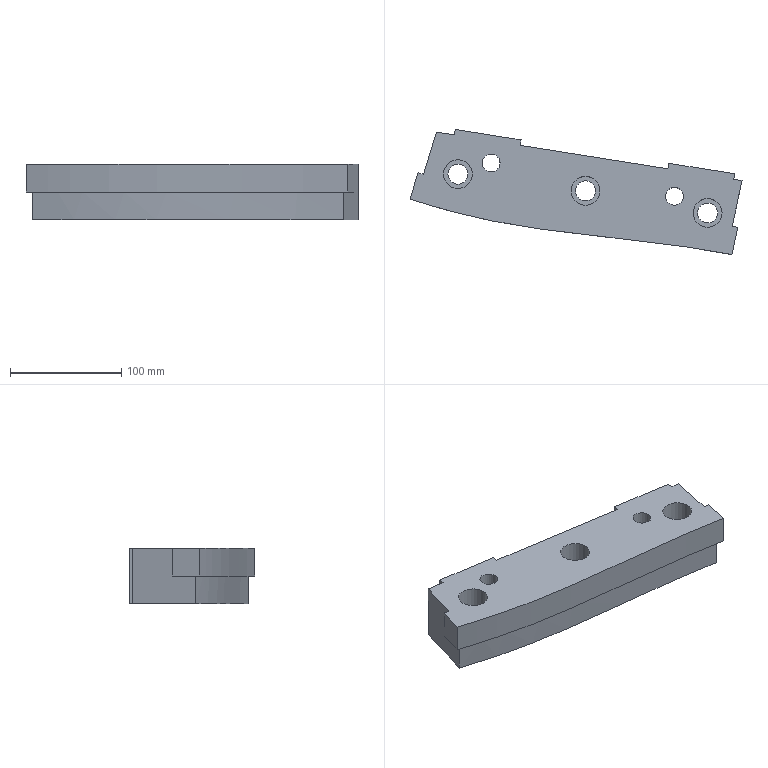Part | NX | features solid 2 | 1 solid | 32 faces | box 299.028 x 112.6 x 50 mm | volume 890723 mm3 | plane 20 | cylinder 8 | spline 4 | commonest cylinder face diameters 18 x3 26 x3 16 x2
STEP:
#1=CARTESIAN_POINT('',(-280.161,-230.257,-25.));
#2=VERTEX_POINT('',#1);
#3=CARTESIAN_POINT('',(-280.161,-230.257,0.));
#4=VERTEX_POINT('',#3);
#5=CARTESIAN_POINT('',(-280.161,-230.257,-25.));
#6=DIRECTION('',(0.,0.,-1.));
#7=VECTOR('',#6,1000.);
#8=LINE('',#5,#7);
#9=EDGE_CURVE('',#2,#4,#8,.F.);
#10=ORIENTED_EDGE('',*,*,#9,.T.);
#11=CARTESIAN_POINT('',(-275.25,-231.199,0.));
#12=VERTEX_POINT('',#11);
#13=CARTESIAN_POINT('',(-275.25,-231.199,0.));
#14=CARTESIAN_POINT('',(-276.886,-230.88,0.));
#15=CARTESIAN_POINT('',(-278.523,-230.565,0.));
#16=CARTESIAN_POINT('',(-280.161,-230.257,0.));
#17=B_SPLINE_CURVE_WITH_KNOTS('',3,(#13,#14,#15,#16),.UNSPECIFIED.,.F.,.F.,(4,4),(1.229,1.234),.UNSPECIFIED.);
#18=EDGE_CURVE('',#12,#4,#17,.T.);
#19=ORIENTED_EDGE('',*,*,#18,.F.);
#20=CARTESIAN_POINT('',(-275.25,-231.199,-25.));
#21=VERTEX_POINT('',#20);
#22=CARTESIAN_POINT('',(-275.25,-231.199,0.));
#23=DIRECTION('',(0.,0.,-1.));
#24=VECTOR('',#23,1000.);
#25=LINE('',#22,#24);
#26=EDGE_CURVE('',#12,#21,#25,.T.);
#27=ORIENTED_EDGE('',*,*,#26,.T.);
#28=CARTESIAN_POINT('',(-275.25,-231.199,-25.));
#29=CARTESIAN_POINT('',(-276.831,-230.891,-25.));
#30=CARTESIAN_POINT('',(-278.519,-230.566,-25.));
#31=CARTESIAN_POINT('',(-280.161,-230.257,-25.));
#32=B_SPLINE_CURVE_WITH_KNOTS('',3,(#28,#29,#30,#31),.UNSPECIFIED.,.F.,.F.,(4,4),(-0.001424,0.01497),.UNSPECIFIED.);
#33=EDGE_CURVE('',#21,#2,#32,.T.);
#34=ORIENTED_EDGE('',*,*,#33,.T.);
#35=EDGE_LOOP('',(#10,#19,#27,#34));
#36=FACE_BOUND('',#35,.T.);
#37=CARTESIAN_POINT('',(-275.25,-231.199,0.));
#38=CARTESIAN_POINT('',(-275.25,-231.199,-25.));
#39=CARTESIAN_POINT('',(-276.831,-230.891,0.));
#40=CARTESIAN_POINT('',(-276.831,-230.891,-25.));
#41=CARTESIAN_POINT('',(-278.519,-230.566,0.));
#42=CARTESIAN_POINT('',(-278.519,-230.566,-25.));
#43=CARTESIAN_POINT('',(-280.161,-230.257,0.));
#44=CARTESIAN_POINT('',(-280.161,-230.257,-25.));
#45=B_SPLINE_SURFACE_WITH_KNOTS('',3,1,((#37,#38),(#39,#40),(#41,#42),(#43,#44)),.SURF_OF_LINEAR_EXTRUSION.,.F.,.F.,.F.,(4,4),(2,2),(-0.001424,0.01497),(0.,1.),.PIECEWISE_BEZIER_KNOTS.);
#46=ADVANCED_FACE('',(#36),#45,.F.);
#47=CARTESIAN_POINT('',(-324.304,-203.241,-50.));
#48=VERTEX_POINT('',#47);
#49=CARTESIAN_POINT('',(-332.304,-203.241,-50.));
#50=DIRECTION('',(0.,0.,1.));
#51=DIRECTION('',(1.,0.,0.));
#52=AXIS2_PLACEMENT_3D('',#49,#50,#51);
#53=CIRCLE('',#52,8.);
#54=EDGE_CURVE('',#48,#48,#53,.F.);
#55=ORIENTED_EDGE('',*,*,#54,.F.);
#56=EDGE_LOOP('',(#55));
#57=FACE_BOUND('',#56,.T.);
#58=CARTESIAN_POINT('',(-489.304,-173.241,-50.));
#59=VERTEX_POINT('',#58);
#60=CARTESIAN_POINT('',(-497.304,-173.241,-50.));
#61=DIRECTION('',(0.,0.,1.));
#62=DIRECTION('',(1.,0.,0.));
#63=AXIS2_PLACEMENT_3D('',#60,#61,#62);
#64=CIRCLE('',#63,8.);
#65=EDGE_CURVE('',#59,#59,#64,.F.);
#66=ORIENTED_EDGE('',*,*,#65,.F.);
#67=EDGE_LOOP('',(#66));
#68=FACE_BOUND('',#67,.T.);
#69=CARTESIAN_POINT('',(-284.32,-249.825,-50.));
#70=VERTEX_POINT('',#69);
#71=CARTESIAN_POINT('',(-271.396,-189.022,-50.));
#72=VERTEX_POINT('',#71);
#73=CARTESIAN_POINT('',(-437.928,-972.492,-50.));
#74=DIRECTION('',(0.2079,0.9781,0.));
#75=VECTOR('',#74,1000.);
#76=LINE('',#73,#75);
#77=EDGE_CURVE('',#70,#72,#76,.T.);
#78=ORIENTED_EDGE('',*,*,#77,.F.);
#79=CARTESIAN_POINT('',(-564.197,-202.638,-50.));
#80=VERTEX_POINT('',#79);
#81=CARTESIAN_POINT('',(-284.32,-249.825,-50.));
#82=CARTESIAN_POINT('',(-287.025,-249.318,-50.));
#83=CARTESIAN_POINT('',(-292.544,-248.318,-50.));
#84=CARTESIAN_POINT('',(-299.718,-247.1,-50.));
#85=CARTESIAN_POINT('',(-305.62,-246.147,-50.));
#86=CARTESIAN_POINT('',(-310.132,-245.441,-50.));
#87=CARTESIAN_POINT('',(-313.95,-244.863,-50.));
#88=CARTESIAN_POINT('',(-316.68,-244.46,-50.));
#89=CARTESIAN_POINT('',(-318.216,-244.236,-50.));
#90=CARTESIAN_POINT('',(-319.469,-244.054,-50.));
#91=CARTESIAN_POINT('',(-320.364,-243.926,-50.));
#92=CARTESIAN_POINT('',(-321.696,-243.736,-50.));
#93=CARTESIAN_POINT('',(-323.997,-243.411,-50.));
#94=CARTESIAN_POINT('',(-328.758,-242.751,-50.));
#95=CARTESIAN_POINT('',(-334.45,-241.992,-50.));
#96=CARTESIAN_POINT('',(-340.417,-241.223,-50.));
#97=CARTESIAN_POINT('',(-344.257,-240.74,-50.));
#98=CARTESIAN_POINT('',(-347.397,-240.351,-50.));
#99=CARTESIAN_POINT('',(-349.387,-240.107,-50.));
#100=CARTESIAN_POINT('',(-350.997,-239.912,-50.));
#101=CARTESIAN_POINT('',(-352.207,-239.765,-50.));
#102=CARTESIAN_POINT('',(-353.243,-239.641,-50.));
#103=CARTESIAN_POINT('',(-354.029,-239.547,-50.));
#104=CARTESIAN_POINT('',(-354.751,-239.46,-50.));
#105=CARTESIAN_POINT('',(-354.973,-239.434,-50.));
#106=CARTESIAN_POINT('',(-355.456,-239.376,-50.));
#107=CARTESIAN_POINT('',(-356.016,-239.31,-50.));
#108=CARTESIAN_POINT('',(-356.743,-239.224,-50.));
#109=CARTESIAN_POINT('',(-357.74,-239.107,-50.));
#110=CARTESIAN_POINT('',(-359.062,-238.952,-50.));
#111=CARTESIAN_POINT('',(-361.325,-238.688,-50.));
#112=CARTESIAN_POINT('',(-364.439,-238.328,-50.));
#113=CARTESIAN_POINT('',(-368.629,-237.847,-50.));
#114=CARTESIAN_POINT('',(-373.272,-237.318,-50.));
#115=CARTESIAN_POINT('',(-378.372,-236.739,-50.));
#116=CARTESIAN_POINT('',(-382.992,-236.217,-50.));
#117=CARTESIAN_POINT('',(-386.441,-235.829,-50.));
#118=CARTESIAN_POINT('',(-388.443,-235.604,-50.));
#119=CARTESIAN_POINT('',(-390.044,-235.424,-50.));
#120=CARTESIAN_POINT('',(-391.403,-235.271,-50.));
#121=CARTESIAN_POINT('',(-393.267,-235.062,-50.));
#122=CARTESIAN_POINT('',(-396.424,-234.705,-50.));
#123=CARTESIAN_POINT('',(-400.758,-234.213,-50.));
#124=CARTESIAN_POINT('',(-405.64,-233.655,-50.));
#125=CARTESIAN_POINT('',(-410.212,-233.127,-50.));
#126=CARTESIAN_POINT('',(-414.473,-232.63,-50.));
#127=CARTESIAN_POINT('',(-417.763,-232.242,-50.));
#128=CARTESIAN_POINT('',(-420.241,-231.947,-50.));
#129=CARTESIAN_POINT('',(-422.018,-231.734,-50.));
#130=CARTESIAN_POINT('',(-423.445,-231.561,-50.));
#131=CARTESIAN_POINT('',(-424.388,-231.446,-50.));
#132=CARTESIAN_POINT('',(-424.951,-231.378,-50.));
#133=CARTESIAN_POINT('',(-425.271,-231.338,-50.));
#134=CARTESIAN_POINT('',(-425.959,-231.254,-50.));
#135=CARTESIAN_POINT('',(-426.745,-231.157,-50.));
#136=CARTESIAN_POINT('',(-428.174,-230.981,-50.));
#137=CARTESIAN_POINT('',(-430.164,-230.732,-50.));
#138=CARTESIAN_POINT('',(-432.535,-230.433,-50.));
#139=CARTESIAN_POINT('',(-435.652,-230.035,-50.));
#140=CARTESIAN_POINT('',(-439.474,-229.538,-50.));
#141=CARTESIAN_POINT('',(-445.427,-228.745,-50.));
#142=CARTESIAN_POINT('',(-451.131,-227.954,-50.));
#143=CARTESIAN_POINT('',(-455.925,-227.262,-50.));
#144=CARTESIAN_POINT('',(-458.249,-226.92,-50.));
#145=CARTESIAN_POINT('',(-459.594,-226.72,-50.));
#146=CARTESIAN_POINT('',(-460.504,-226.583,-50.));
#147=CARTESIAN_POINT('',(-461.755,-226.394,-50.));
#148=CARTESIAN_POINT('',(-463.295,-226.159,-50.));
#149=CARTESIAN_POINT('',(-466.028,-225.737,-50.));
#150=CARTESIAN_POINT('',(-469.846,-225.132,-50.));
#151=CARTESIAN_POINT('',(-474.352,-224.394,-50.));
#152=CARTESIAN_POINT('',(-480.236,-223.396,-50.));
#153=CARTESIAN_POINT('',(-485.951,-222.374,-50.));
#154=CARTESIAN_POINT('',(-490.776,-221.466,-50.));
#155=CARTESIAN_POINT('',(-493.518,-220.935,-50.));
#156=CARTESIAN_POINT('',(-495.471,-220.551,-50.));
#157=CARTESIAN_POINT('',(-497.714,-220.101,-50.));
#158=CARTESIAN_POINT('',(-500.598,-219.511,-50.));
#159=CARTESIAN_POINT('',(-505.683,-218.44,-50.));
#160=CARTESIAN_POINT('',(-512.89,-216.834,-50.));
#161=CARTESIAN_POINT('',(-520.076,-215.115,-50.));
#162=CARTESIAN_POINT('',(-525.782,-213.68,-50.));
#163=CARTESIAN_POINT('',(-530.098,-212.558,-50.));
#164=CARTESIAN_POINT('',(-534.215,-211.455,-50.));
#165=CARTESIAN_POINT('',(-538.494,-210.276,-50.));
#166=CARTESIAN_POINT('',(-542.88,-209.036,-50.));
#167=CARTESIAN_POINT('',(-551.585,-206.518,-50.));
#168=CARTESIAN_POINT('',(-558.639,-204.383,-50.));
#169=CARTESIAN_POINT('',(-564.197,-202.638,-50.));
#170=B_SPLINE_CURVE_WITH_KNOTS('',3,(#81,#82,#83,#84,#85,#86,#87,#88,#89,#90,#91,#92,#93,#94,#95,#96,#97,#98,#99,#100,#101,#102,#103,#104,#105,#106,#107,#108,#109,#110,#111,#112,#113,#114,#115,#116,#117,#118,#119,#120,#121,#122,#123,#124,#125,#126,#127,#128,#129,#130,#131,#132,#133,#134,#135,#136,#137,#138,#139,#140,#141,#142,#143,#144,#145,#146,#147,#148,#149,#150,#151,#152,#153,#154,#155,#156,#157,#158,#159,#160,#161,#162,#163,#164,#165,#166,#167,#168,#169),.UNSPECIFIED.,.F.,.F.,(4,1,1,1,1,1,1,1,1,1,1,1,1,1,1,1,1,1,1,1,1,1,1,1,1,1,1,1,1,1,1,1,1,1,1,1,1,1,1,1,1,1,1,1,1,1,1,1,1,1,1,1,1,1,1,1,1,1,1,1,1,1,1,1,1,1,1,1,1,1,1,1,1,1,1,1,1,1,1,1,1,1,1,1,1,1,4),(0.,0.03125,0.0625,0.07812,0.09375,0.1094,0.1172,0.1211,0.125,0.1289,0.1328,0.1406,0.1562,0.1875,0.2031,0.2188,0.2266,0.2344,0.2383,0.2422,0.2461,0.248,0.25,0.252,0.2539,0.2578,0.2617,0.2656,0.2734,0.2812,0.2969,0.3125,0.3281,0.3438,0.3594,0.3672,0.3711,0.375,0.3789,0.3828,0.3906,0.4062,0.4219,0.4375,0.4531,0.4688,0.4766,0.4844,0.4922,0.4961,0.498,0.5,0.502,0.5039,0.5078,0.5156,0.5234,0.5312,0.5469,0.5625,0.5938,0.6094,0.6172,0.6211,0.625,0.6289,0.6328,0.6406,0.6562,0.6719,0.6875,0.7188,0.7344,0.7422,0.75,0.7578,0.7656,0.7812,0.8125,0.8438,0.8594,0.875,0.8906,0.9062,0.9219,0.9375,1.),.UNSPECIFIED.);
#171=EDGE_CURVE('',#70,#80,#170,.T.);
#172=ORIENTED_EDGE('',*,*,#171,.T.);
#173=CARTESIAN_POINT('',(-546.703,-145.418,-50.));
#174=VERTEX_POINT('',#173);
#175=CARTESIAN_POINT('',(-769.978,-875.717,-50.));
#176=DIRECTION('',(0.2924,0.9563,0.));
#177=VECTOR('',#176,1000.);
#178=LINE('',#175,#177);
#179=EDGE_CURVE('',#80,#174,#178,.T.);
#180=ORIENTED_EDGE('',*,*,#179,.T.);
#181=CARTESIAN_POINT('',(-530.432,-147.995,-50.));
#182=VERTEX_POINT('',#181);
#183=CARTESIAN_POINT('',(-364.132,-174.334,-50.));
#184=DIRECTION('',(0.9877,-0.1564,0.));
#185=VECTOR('',#184,1000.);
#186=LINE('',#183,#185);
#187=EDGE_CURVE('',#174,#182,#186,.T.);
#188=ORIENTED_EDGE('',*,*,#187,.T.);
#189=CARTESIAN_POINT('',(-529.65,-143.056,-50.));
#190=VERTEX_POINT('',#189);
#191=CARTESIAN_POINT('',(-528.086,-133.179,-50.));
#192=DIRECTION('',(0.1564,0.9877,0.));
#193=VECTOR('',#192,1000.);
#194=LINE('',#191,#193);
#195=EDGE_CURVE('',#182,#190,#194,.T.);
#196=ORIENTED_EDGE('',*,*,#195,.T.);
#197=CARTESIAN_POINT('',(-470.389,-152.442,-50.));
#198=VERTEX_POINT('',#197);
#199=CARTESIAN_POINT('',(-363.35,-169.396,-50.));
#200=DIRECTION('',(0.9877,-0.1564,0.));
#201=VECTOR('',#200,1000.);
#202=LINE('',#199,#201);
#203=EDGE_CURVE('',#190,#198,#202,.T.);
#204=ORIENTED_EDGE('',*,*,#203,.T.);
#205=CARTESIAN_POINT('',(-471.171,-157.381,-50.));
#206=VERTEX_POINT('',#205);
#207=CARTESIAN_POINT('',(-468.825,-142.565,-50.));
#208=DIRECTION('',(0.1564,0.9877,0.));
#209=VECTOR('',#208,1000.);
#210=LINE('',#207,#209);
#211=EDGE_CURVE('',#206,#198,#210,.T.);
#212=ORIENTED_EDGE('',*,*,#211,.F.);
#213=CARTESIAN_POINT('',(-338.153,-178.449,-50.));
#214=VERTEX_POINT('',#213);
#215=CARTESIAN_POINT('',(-364.132,-174.334,-50.));
#216=DIRECTION('',(0.9877,-0.1564,0.));
#217=VECTOR('',#216,1000.);
#218=LINE('',#215,#217);
#219=EDGE_CURVE('',#206,#214,#218,.T.);
#220=ORIENTED_EDGE('',*,*,#219,.T.);
#221=CARTESIAN_POINT('',(-337.371,-173.51,-50.));
#222=VERTEX_POINT('',#221);
#223=CARTESIAN_POINT('',(-335.807,-163.633,-50.));
#224=DIRECTION('',(0.1564,0.9877,0.));
#225=VECTOR('',#224,1000.);
#226=LINE('',#223,#225);
#227=EDGE_CURVE('',#214,#222,#226,.T.);
#228=ORIENTED_EDGE('',*,*,#227,.T.);
#229=CARTESIAN_POINT('',(-278.11,-182.896,-50.));
#230=VERTEX_POINT('',#229);
#231=CARTESIAN_POINT('',(-363.35,-169.396,-50.));
#232=DIRECTION('',(0.9877,-0.1564,0.));
#233=VECTOR('',#232,1000.);
#234=LINE('',#231,#233);
#235=EDGE_CURVE('',#222,#230,#234,.T.);
#236=ORIENTED_EDGE('',*,*,#235,.T.);
#237=CARTESIAN_POINT('',(-278.892,-187.835,-50.));
#238=VERTEX_POINT('',#237);
#239=CARTESIAN_POINT('',(-276.545,-173.019,-50.));
#240=DIRECTION('',(0.1564,0.9877,0.));
#241=VECTOR('',#240,1000.);
#242=LINE('',#239,#241);
#243=EDGE_CURVE('',#238,#230,#242,.T.);
#244=ORIENTED_EDGE('',*,*,#243,.F.);
#245=CARTESIAN_POINT('',(-364.132,-174.334,-50.));
#246=DIRECTION('',(0.9877,-0.1564,0.));
#247=VECTOR('',#246,1000.);
#248=LINE('',#245,#247);
#249=EDGE_CURVE('',#238,#72,#248,.T.);
#250=ORIENTED_EDGE('',*,*,#249,.T.);
#251=EDGE_LOOP('',(#78,#172,#180,#188,#196,#204,#212,#220,#228,#236,#244,#250));
#252=FACE_BOUND('',#251,.T.);
#253=CARTESIAN_POINT('',(-518.304,-183.241,-50.));
#254=VERTEX_POINT('',#253);
#255=CARTESIAN_POINT('',(-527.304,-183.241,-50.));
#256=DIRECTION('',(0.,0.,1.));
#257=DIRECTION('',(1.,0.,0.));
#258=AXIS2_PLACEMENT_3D('',#255,#256,#257);
#259=CIRCLE('',#258,9.);
#260=EDGE_CURVE('',#254,#254,#259,.F.);
#261=ORIENTED_EDGE('',*,*,#260,.F.);
#262=EDGE_LOOP('',(#261));
#263=FACE_BOUND('',#262,.T.);
#264=CARTESIAN_POINT('',(-403.304,-198.241,-50.));
#265=VERTEX_POINT('',#264);
#266=CARTESIAN_POINT('',(-412.304,-198.241,-50.));
#267=DIRECTION('',(0.,0.,1.));
#268=DIRECTION('',(1.,0.,0.));
#269=AXIS2_PLACEMENT_3D('',#266,#267,#268);
#270=CIRCLE('',#269,9.);
#271=EDGE_CURVE('',#265,#265,#270,.F.);
#272=ORIENTED_EDGE('',*,*,#271,.F.);
#273=EDGE_LOOP('',(#272));
#274=FACE_BOUND('',#273,.T.);
#275=CARTESIAN_POINT('',(-293.304,-218.241,-50.));
#276=VERTEX_POINT('',#275);
#277=CARTESIAN_POINT('',(-302.304,-218.241,-50.));
#278=DIRECTION('',(0.,0.,1.));
#279=DIRECTION('',(1.,0.,0.));
#280=AXIS2_PLACEMENT_3D('',#277,#278,#279);
#281=CIRCLE('',#280,9.);
#282=EDGE_CURVE('',#276,#276,#281,.F.);
#283=ORIENTED_EDGE('',*,*,#282,.F.);
#284=EDGE_LOOP('',(#283));
#285=FACE_BOUND('',#284,.T.);
#286=CARTESIAN_POINT('',(-488.834,-961.671,-50.));
#287=DIRECTION('',(0.,0.,1.));
#288=DIRECTION('',(1.,0.,0.));
#289=AXIS2_PLACEMENT_3D('',#286,#287,#288);
#290=PLANE('',#289);
#291=ADVANCED_FACE('',(#57,#68,#252,#263,#274,#285),#290,.F.);
#292=CARTESIAN_POINT('',(-338.153,-178.449,0.));
#293=VERTEX_POINT('',#292);
#294=CARTESIAN_POINT('',(-338.153,-178.449,-25.));
#295=DIRECTION('',(0.,0.,-1.));
#296=VECTOR('',#295,1000.);
#297=LINE('',#294,#296);
#298=EDGE_CURVE('',#293,#214,#297,.T.);
#299=ORIENTED_EDGE('',*,*,#298,.T.);
#300=ORIENTED_EDGE('',*,*,#219,.F.);
#301=CARTESIAN_POINT('',(-471.171,-157.381,0.));
#302=VERTEX_POINT('',#301);
#303=CARTESIAN_POINT('',(-471.171,-157.381,-25.));
#304=DIRECTION('',(0.,0.,-1.));
#305=VECTOR('',#304,1000.);
#306=LINE('',#303,#305);
#307=EDGE_CURVE('',#302,#206,#306,.T.);
#308=ORIENTED_EDGE('',*,*,#307,.F.);
#309=CARTESIAN_POINT('',(-612.069,-135.065,0.));
#310=DIRECTION('',(-0.9877,0.1564,0.));
#311=VECTOR('',#310,1000.);
#312=LINE('',#309,#311);
#313=EDGE_CURVE('',#293,#302,#312,.T.);
#314=ORIENTED_EDGE('',*,*,#313,.F.);
#315=EDGE_LOOP('',(#299,#300,#308,#314));
#316=FACE_BOUND('',#315,.T.);
#317=CARTESIAN_POINT('',(-612.069,-135.065,-70.));
#318=DIRECTION('',(-0.1564,-0.9877,0.));
#319=DIRECTION('',(0.9877,-0.1564,0.));
#320=AXIS2_PLACEMENT_3D('',#317,#318,#319);
#321=PLANE('',#320);
#322=ADVANCED_FACE('',(#316),#321,.F.);
#323=CARTESIAN_POINT('',(-530.432,-147.995,0.));
#324=VERTEX_POINT('',#323);
#325=CARTESIAN_POINT('',(-530.432,-147.995,-25.));
#326=DIRECTION('',(0.,0.,-1.));
#327=VECTOR('',#326,1000.);
#328=LINE('',#325,#327);
#329=EDGE_CURVE('',#324,#182,#328,.T.);
#330=ORIENTED_EDGE('',*,*,#329,.T.);
#331=ORIENTED_EDGE('',*,*,#187,.F.);
#332=CARTESIAN_POINT('',(-546.703,-145.418,0.));
#333=VERTEX_POINT('',#332);
#334=CARTESIAN_POINT('',(-546.703,-145.418,-70.));
#335=DIRECTION('',(0.,0.,1.));
#336=VECTOR('',#335,1000.);
#337=LINE('',#334,#336);
#338=EDGE_CURVE('',#174,#333,#337,.T.);
#339=ORIENTED_EDGE('',*,*,#338,.T.);
#340=CARTESIAN_POINT('',(-612.069,-135.065,0.));
#341=DIRECTION('',(-0.9877,0.1564,0.));
#342=VECTOR('',#341,1000.);
#343=LINE('',#340,#342);
#344=EDGE_CURVE('',#324,#333,#343,.T.);
#345=ORIENTED_EDGE('',*,*,#344,.F.);
#346=EDGE_LOOP('',(#330,#331,#339,#345));
#347=FACE_BOUND('',#346,.T.);
#348=CARTESIAN_POINT('',(-612.069,-135.065,-70.));
#349=DIRECTION('',(-0.1564,-0.9877,0.));
#350=DIRECTION('',(0.9877,-0.1564,0.));
#351=AXIS2_PLACEMENT_3D('',#348,#349,#350);
#352=PLANE('',#351);
#353=ADVANCED_FACE('',(#347),#352,.F.);
#354=ORIENTED_EDGE('',*,*,#249,.F.);
#355=CARTESIAN_POINT('',(-278.892,-187.835,0.));
#356=VERTEX_POINT('',#355);
#357=CARTESIAN_POINT('',(-278.892,-187.835,-25.));
#358=DIRECTION('',(0.,0.,-1.));
#359=VECTOR('',#358,1000.);
#360=LINE('',#357,#359);
#361=EDGE_CURVE('',#356,#238,#360,.T.);
#362=ORIENTED_EDGE('',*,*,#361,.F.);
#363=CARTESIAN_POINT('',(-271.396,-189.022,0.));
#364=VERTEX_POINT('',#363);
#365=CARTESIAN_POINT('',(-612.069,-135.065,0.));
#366=DIRECTION('',(-0.9877,0.1564,0.));
#367=VECTOR('',#366,1000.);
#368=LINE('',#365,#367);
#369=EDGE_CURVE('',#364,#356,#368,.T.);
#370=ORIENTED_EDGE('',*,*,#369,.F.);
#371=CARTESIAN_POINT('',(-271.396,-189.022,-70.));
#372=DIRECTION('',(0.,0.,1.));
#373=VECTOR('',#372,1000.);
#374=LINE('',#371,#373);
#375=EDGE_CURVE('',#72,#364,#374,.T.);
#376=ORIENTED_EDGE('',*,*,#375,.F.);
#377=EDGE_LOOP('',(#354,#362,#370,#376));
#378=FACE_BOUND('',#377,.T.);
#379=CARTESIAN_POINT('',(-612.069,-135.065,-70.));
#380=DIRECTION('',(-0.1564,-0.9877,0.));
#381=DIRECTION('',(0.9877,-0.1564,0.));
#382=AXIS2_PLACEMENT_3D('',#379,#380,#381);
#383=PLANE('',#382);
#384=ADVANCED_FACE('',(#378),#383,.F.);
#385=CARTESIAN_POINT('',(-563.114,-181.994,0.));
#386=VERTEX_POINT('',#385);
#387=CARTESIAN_POINT('',(-562.751,-182.111,0.));
#388=VERTEX_POINT('',#387);
#389=CARTESIAN_POINT('',(-268.069,-277.149,0.));
#390=DIRECTION('',(0.9517,-0.3069,0.));
#391=VECTOR('',#390,1000.);
#392=LINE('',#389,#391);
#393=EDGE_CURVE('',#386,#388,#392,.T.);
#394=ORIENTED_EDGE('',*,*,#393,.F.);
#395=CARTESIAN_POINT('',(-570.424,-205.904,0.));
#396=VERTEX_POINT('',#395);
#397=CARTESIAN_POINT('',(-774.76,-874.255,0.));
#398=DIRECTION('',(0.2924,0.9563,0.));
#399=VECTOR('',#398,1000.);
#400=LINE('',#397,#399);
#401=EDGE_CURVE('',#396,#386,#400,.T.);
#402=ORIENTED_EDGE('',*,*,#401,.F.);
#403=CARTESIAN_POINT('',(-280.448,-255.656,0.));
#404=VERTEX_POINT('',#403);
#405=CARTESIAN_POINT('',(-280.448,-255.656,0.));
#406=CARTESIAN_POINT('',(-304.601,-250.945,0.));
#407=CARTESIAN_POINT('',(-353.317,-244.246,0.));
#408=CARTESIAN_POINT('',(-414.5,-237.947,0.));
#409=CARTESIAN_POINT('',(-463.256,-231.458,0.));
#410=CARTESIAN_POINT('',(-499.498,-225.232,0.));
#411=CARTESIAN_POINT('',(-529.277,-218.168,0.));
#412=CARTESIAN_POINT('',(-552.84,-211.384,0.));
#413=CARTESIAN_POINT('',(-564.576,-207.79,0.));
#414=CARTESIAN_POINT('',(-570.424,-205.904,0.));
#415=B_SPLINE_CURVE_WITH_KNOTS('',3,(#405,#406,#407,#408,#409,#410,#411,#412,#413,#414),.UNSPECIFIED.,.F.,.F.,(4,1,1,1,1,1,1,4),(0.3905,0.4642,0.5379,0.5748,0.6116,0.6485,0.6669,0.6853),.UNSPECIFIED.);
#416=EDGE_CURVE('',#404,#396,#415,.T.);
#417=ORIENTED_EDGE('',*,*,#416,.F.);
#418=CARTESIAN_POINT('',(-433.037,-973.531,0.));
#419=DIRECTION('',(0.2079,0.9781,0.));
#420=VECTOR('',#419,1000.);
#421=LINE('',#418,#420);
#422=EDGE_CURVE('',#404,#12,#421,.T.);
#423=ORIENTED_EDGE('',*,*,#422,.T.);
#424=ORIENTED_EDGE('',*,*,#18,.T.);
#425=CARTESIAN_POINT('',(-284.299,-249.725,0.));
#426=DIRECTION('',(-0.2079,-0.9781,0.));
#427=VECTOR('',#426,1000.);
#428=LINE('',#425,#427);
#429=EDGE_CURVE('',#364,#4,#428,.T.);
#430=ORIENTED_EDGE('',*,*,#429,.F.);
#431=ORIENTED_EDGE('',*,*,#369,.T.);
#432=CARTESIAN_POINT('',(-278.11,-182.896,0.));
#433=VERTEX_POINT('',#432);
#434=CARTESIAN_POINT('',(-289.409,-254.237,0.));
#435=DIRECTION('',(0.1564,0.9877,0.));
#436=VECTOR('',#435,1000.);
#437=LINE('',#434,#436);
#438=EDGE_CURVE('',#356,#433,#437,.T.);
#439=ORIENTED_EDGE('',*,*,#438,.T.);
#440=CARTESIAN_POINT('',(-337.371,-173.51,0.));
#441=VERTEX_POINT('',#440);
#442=CARTESIAN_POINT('',(-363.35,-169.396,0.));
#443=DIRECTION('',(0.9877,-0.1564,0.));
#444=VECTOR('',#443,1000.);
#445=LINE('',#442,#444);
#446=EDGE_CURVE('',#441,#433,#445,.T.);
#447=ORIENTED_EDGE('',*,*,#446,.F.);
#448=CARTESIAN_POINT('',(-348.67,-244.851,0.));
#449=DIRECTION('',(0.1564,0.9877,0.));
#450=VECTOR('',#449,1000.);
#451=LINE('',#448,#450);
#452=EDGE_CURVE('',#293,#441,#451,.T.);
#453=ORIENTED_EDGE('',*,*,#452,.F.);
#454=ORIENTED_EDGE('',*,*,#313,.T.);
#455=CARTESIAN_POINT('',(-470.389,-152.442,0.));
#456=VERTEX_POINT('',#455);
#457=CARTESIAN_POINT('',(-481.688,-223.783,0.));
#458=DIRECTION('',(0.1564,0.9877,0.));
#459=VECTOR('',#458,1000.);
#460=LINE('',#457,#459);
#461=EDGE_CURVE('',#302,#456,#460,.T.);
#462=ORIENTED_EDGE('',*,*,#461,.T.);
#463=CARTESIAN_POINT('',(-529.65,-143.056,0.));
#464=VERTEX_POINT('',#463);
#465=CARTESIAN_POINT('',(-363.35,-169.396,0.));
#466=DIRECTION('',(0.9877,-0.1564,0.));
#467=VECTOR('',#466,1000.);
#468=LINE('',#465,#467);
#469=EDGE_CURVE('',#464,#456,#468,.T.);
#470=ORIENTED_EDGE('',*,*,#469,.F.);
#471=CARTESIAN_POINT('',(-540.95,-214.397,0.));
#472=DIRECTION('',(0.1564,0.9877,0.));
#473=VECTOR('',#472,1000.);
#474=LINE('',#471,#473);
#475=EDGE_CURVE('',#324,#464,#474,.T.);
#476=ORIENTED_EDGE('',*,*,#475,.F.);
#477=ORIENTED_EDGE('',*,*,#344,.T.);
#478=CARTESIAN_POINT('',(-558.35,-183.512,0.));
#479=VERTEX_POINT('',#478);
#480=CARTESIAN_POINT('',(-564.181,-202.584,0.));
#481=DIRECTION('',(-0.2924,-0.9563,0.));
#482=VECTOR('',#481,1000.);
#483=LINE('',#480,#482);
#484=EDGE_CURVE('',#333,#479,#483,.T.);
#485=ORIENTED_EDGE('',*,*,#484,.T.);
#486=CARTESIAN_POINT('',(-558.35,-183.512,0.));
#487=CARTESIAN_POINT('',(-559.818,-183.05,0.));
#488=CARTESIAN_POINT('',(-561.285,-182.584,0.));
#489=CARTESIAN_POINT('',(-562.751,-182.111,0.));
#490=B_SPLINE_CURVE_WITH_KNOTS('',3,(#486,#487,#488,#489),.UNSPECIFIED.,.F.,.F.,(4,4),(1.517,1.521),.UNSPECIFIED.);
#491=EDGE_CURVE('',#479,#388,#490,.T.);
#492=ORIENTED_EDGE('',*,*,#491,.T.);
#493=EDGE_LOOP('',(#394,#402,#417,#423,#424,#430,#431,#439,#447,#453,#454,#462,#470,#476,#477,#485,#492));
#494=FACE_BOUND('',#493,.T.);
#495=CARTESIAN_POINT('',(-399.304,-198.241,0.));
#496=VERTEX_POINT('',#495);
#497=CARTESIAN_POINT('',(-412.304,-198.241,0.));
#498=DIRECTION('',(0.,0.,1.));
#499=DIRECTION('',(1.,0.,0.));
#500=AXIS2_PLACEMENT_3D('',#497,#498,#499);
#501=CIRCLE('',#500,13.);
#502=EDGE_CURVE('',#496,#496,#501,.F.);
#503=ORIENTED_EDGE('',*,*,#502,.T.);
#504=EDGE_LOOP('',(#503));
#505=FACE_BOUND('',#504,.T.);
#506=CARTESIAN_POINT('',(-489.304,-173.241,0.));
#507=VERTEX_POINT('',#506);
#508=CARTESIAN_POINT('',(-497.304,-173.241,0.));
#509=DIRECTION('',(0.,0.,1.));
#510=DIRECTION('',(1.,0.,0.));
#511=AXIS2_PLACEMENT_3D('',#508,#509,#510);
#512=CIRCLE('',#511,8.);
#513=EDGE_CURVE('',#507,#507,#512,.F.);
#514=ORIENTED_EDGE('',*,*,#513,.T.);
#515=EDGE_LOOP('',(#514));
#516=FACE_BOUND('',#515,.T.);
#517=CARTESIAN_POINT('',(-324.304,-203.241,0.));
#518=VERTEX_POINT('',#517);
#519=CARTESIAN_POINT('',(-332.304,-203.241,0.));
#520=DIRECTION('',(0.,0.,1.));
#521=DIRECTION('',(1.,0.,0.));
#522=AXIS2_PLACEMENT_3D('',#519,#520,#521);
#523=CIRCLE('',#522,8.);
#524=EDGE_CURVE('',#518,#518,#523,.F.);
#525=ORIENTED_EDGE('',*,*,#524,.T.);
#526=EDGE_LOOP('',(#525));
#527=FACE_BOUND('',#526,.T.);
#528=CARTESIAN_POINT('',(-514.304,-183.241,0.));
#529=VERTEX_POINT('',#528);
#530=CARTESIAN_POINT('',(-527.304,-183.241,0.));
#531=DIRECTION('',(0.,0.,1.));
#532=DIRECTION('',(1.,0.,0.));
#533=AXIS2_PLACEMENT_3D('',#530,#531,#532);
#534=CIRCLE('',#533,13.);
#535=EDGE_CURVE('',#529,#529,#534,.F.);
#536=ORIENTED_EDGE('',*,*,#535,.T.);
#537=EDGE_LOOP('',(#536));
#538=FACE_BOUND('',#537,.T.);
#539=CARTESIAN_POINT('',(-289.304,-218.241,0.));
#540=VERTEX_POINT('',#539);
#541=CARTESIAN_POINT('',(-302.304,-218.241,0.));
#542=DIRECTION('',(0.,0.,1.));
#543=DIRECTION('',(1.,0.,0.));
#544=AXIS2_PLACEMENT_3D('',#541,#542,#543);
#545=CIRCLE('',#544,13.);
#546=EDGE_CURVE('',#540,#540,#545,.F.);
#547=ORIENTED_EDGE('',*,*,#546,.T.);
#548=EDGE_LOOP('',(#547));
#549=FACE_BOUND('',#548,.T.);
#550=CARTESIAN_POINT('',(-488.834,-961.671,0.));
#551=DIRECTION('',(0.,0.,1.));
#552=DIRECTION('',(1.,0.,0.));
#553=AXIS2_PLACEMENT_3D('',#550,#551,#552);
#554=PLANE('',#553);
#555=ADVANCED_FACE('',(#494,#505,#516,#527,#538,#549),#554,.T.);
#556=CARTESIAN_POINT('',(-563.114,-181.994,-25.));
#557=VERTEX_POINT('',#556);
#558=CARTESIAN_POINT('',(-562.751,-182.111,-25.));
#559=VERTEX_POINT('',#558);
#560=CARTESIAN_POINT('',(-600.82,-169.834,-25.));
#561=DIRECTION('',(0.9517,-0.3069,0.));
#562=VECTOR('',#561,1000.);
#563=LINE('',#560,#562);
#564=EDGE_CURVE('',#557,#559,#563,.T.);
#565=ORIENTED_EDGE('',*,*,#564,.T.);
#566=CARTESIAN_POINT('',(-558.35,-183.512,-25.));
#567=VERTEX_POINT('',#566);
#568=CARTESIAN_POINT('',(-558.35,-183.512,-25.));
#569=CARTESIAN_POINT('',(-559.823,-183.049,-25.));
#570=CARTESIAN_POINT('',(-561.29,-182.582,-25.));
#571=CARTESIAN_POINT('',(-562.751,-182.111,-25.));
#572=B_SPLINE_CURVE_WITH_KNOTS('',3,(#568,#569,#570,#571),.UNSPECIFIED.,.F.,.F.,(4,4),(0.9837,1.),.UNSPECIFIED.);
#573=EDGE_CURVE('',#567,#559,#572,.T.);
#574=ORIENTED_EDGE('',*,*,#573,.F.);
#575=CARTESIAN_POINT('',(-564.197,-202.638,-25.));
#576=VERTEX_POINT('',#575);
#577=CARTESIAN_POINT('',(-564.181,-202.584,-25.));
#578=DIRECTION('',(0.2924,0.9563,0.));
#579=VECTOR('',#578,1000.);
#580=LINE('',#577,#579);
#581=EDGE_CURVE('',#576,#567,#580,.T.);
#582=ORIENTED_EDGE('',*,*,#581,.F.);
#583=CARTESIAN_POINT('',(-284.32,-249.825,-25.));
#584=VERTEX_POINT('',#583);
#585=CARTESIAN_POINT('',(-284.32,-249.825,-25.));
#586=CARTESIAN_POINT('',(-307.639,-245.454,-25.));
#587=CARTESIAN_POINT('',(-354.608,-239.106,-25.));
#588=CARTESIAN_POINT('',(-413.551,-233.,-25.));
#589=CARTESIAN_POINT('',(-460.518,-226.792,-25.));
#590=CARTESIAN_POINT('',(-495.563,-220.896,-25.));
#591=CARTESIAN_POINT('',(-530.208,-212.894,-25.));
#592=CARTESIAN_POINT('',(-552.9,-206.185,-25.));
#593=CARTESIAN_POINT('',(-564.197,-202.638,-25.));
#594=B_SPLINE_CURVE_WITH_KNOTS('',3,(#585,#586,#587,#588,#589,#590,#591,#592,#593),.UNSPECIFIED.,.F.,.F.,(4,1,1,1,1,1,4),(1.211,1.282,1.353,1.389,1.425,1.46,1.496),.UNSPECIFIED.);
#595=EDGE_CURVE('',#584,#576,#594,.T.);
#596=ORIENTED_EDGE('',*,*,#595,.F.);
#597=CARTESIAN_POINT('',(-284.299,-249.725,-25.));
#598=DIRECTION('',(0.2079,0.9781,0.));
#599=VECTOR('',#598,1000.);
#600=LINE('',#597,#599);
#601=EDGE_CURVE('',#584,#2,#600,.T.);
#602=ORIENTED_EDGE('',*,*,#601,.T.);
#603=ORIENTED_EDGE('',*,*,#33,.F.);
#604=CARTESIAN_POINT('',(-280.448,-255.656,-25.));
#605=VERTEX_POINT('',#604);
#606=CARTESIAN_POINT('',(-578.39,-1657.361,-25.));
#607=DIRECTION('',(0.2079,0.9781,0.));
#608=VECTOR('',#607,1000.);
#609=LINE('',#606,#608);
#610=EDGE_CURVE('',#605,#21,#609,.T.);
#611=ORIENTED_EDGE('',*,*,#610,.F.);
#612=CARTESIAN_POINT('',(-570.424,-205.904,-25.));
#613=VERTEX_POINT('',#612);
#614=CARTESIAN_POINT('',(-280.448,-255.656,-25.));
#615=CARTESIAN_POINT('',(-304.618,-250.942,-25.));
#616=CARTESIAN_POINT('',(-353.344,-244.243,-25.));
#617=CARTESIAN_POINT('',(-414.567,-237.939,-25.));
#618=CARTESIAN_POINT('',(-463.297,-231.451,-25.));
#619=CARTESIAN_POINT('',(-499.525,-225.226,-25.));
#620=CARTESIAN_POINT('',(-529.292,-218.164,-25.));
#621=CARTESIAN_POINT('',(-552.847,-211.382,-25.));
#622=CARTESIAN_POINT('',(-564.579,-207.79,-25.));
#623=CARTESIAN_POINT('',(-570.424,-205.904,-25.));
#624=B_SPLINE_CURVE_WITH_KNOTS('',3,(#614,#615,#616,#617,#618,#619,#620,#621,#622,#623),.UNSPECIFIED.,.F.,.F.,(4,1,1,1,1,1,1,4),(0.4066,0.4805,0.5543,0.5913,0.6282,0.6651,0.6836,0.7021),.UNSPECIFIED.);
#625=EDGE_CURVE('',#605,#613,#624,.T.);
#626=ORIENTED_EDGE('',*,*,#625,.T.);
#627=CARTESIAN_POINT('',(-976.675,-1534.691,-25.));
#628=DIRECTION('',(0.2924,0.9563,0.));
#629=VECTOR('',#628,1000.);
#630=LINE('',#627,#629);
#631=EDGE_CURVE('',#613,#557,#630,.T.);
#632=ORIENTED_EDGE('',*,*,#631,.T.);
#633=EDGE_LOOP('',(#565,#574,#582,#596,#602,#603,#611,#626,#632));
#634=FACE_BOUND('',#633,.T.);
#635=CARTESIAN_POINT('',(-280.448,-255.656,-25.));
#636=DIRECTION('',(0.,0.,-1.));
#637=DIRECTION('',(-1.,0.,0.));
#638=AXIS2_PLACEMENT_3D('',#635,#636,#637);
#639=PLANE('',#638);
#640=ADVANCED_FACE('',(#634),#639,.T.);
#641=ORIENTED_EDGE('',*,*,#338,.F.);
#642=ORIENTED_EDGE('',*,*,#179,.F.);
#643=CARTESIAN_POINT('',(-564.197,-202.638,-42.5));
#644=DIRECTION('',(0.,0.,1.));
#645=VECTOR('',#644,1000.);
#646=LINE('',#643,#645);
#647=EDGE_CURVE('',#80,#576,#646,.T.);
#648=ORIENTED_EDGE('',*,*,#647,.T.);
#649=ORIENTED_EDGE('',*,*,#581,.T.);
#650=CARTESIAN_POINT('',(-558.35,-183.512,-25.));
#651=DIRECTION('',(0.,0.,-1.));
#652=VECTOR('',#651,1000.);
#653=LINE('',#650,#652);
#654=EDGE_CURVE('',#567,#479,#653,.F.);
#655=ORIENTED_EDGE('',*,*,#654,.T.);
#656=ORIENTED_EDGE('',*,*,#484,.F.);
#657=EDGE_LOOP('',(#641,#642,#648,#649,#655,#656));
#658=FACE_BOUND('',#657,.T.);
#659=CARTESIAN_POINT('',(-564.181,-202.584,-70.));
#660=DIRECTION('',(0.9563,-0.2924,0.));
#661=DIRECTION('',(0.2924,0.9563,0.));
#662=AXIS2_PLACEMENT_3D('',#659,#660,#661);
#663=PLANE('',#662);
#664=ADVANCED_FACE('',(#658),#663,.F.);
#665=ORIENTED_EDGE('',*,*,#375,.T.);
#666=ORIENTED_EDGE('',*,*,#429,.T.);
#667=ORIENTED_EDGE('',*,*,#9,.F.);
#668=ORIENTED_EDGE('',*,*,#601,.F.);
#669=CARTESIAN_POINT('',(-284.32,-249.825,-42.5));
#670=DIRECTION('',(0.,0.,1.));
#671=VECTOR('',#670,1000.);
#672=LINE('',#669,#671);
#673=EDGE_CURVE('',#70,#584,#672,.T.);
#674=ORIENTED_EDGE('',*,*,#673,.F.);
#675=ORIENTED_EDGE('',*,*,#77,.T.);
#676=EDGE_LOOP('',(#665,#666,#667,#668,#674,#675));
#677=FACE_BOUND('',#676,.T.);
#678=CARTESIAN_POINT('',(-284.299,-249.725,-70.));
#679=DIRECTION('',(0.9781,-0.2079,0.));
#680=DIRECTION('',(0.2079,0.9781,0.));
#681=AXIS2_PLACEMENT_3D('',#678,#679,#680);
#682=PLANE('',#681);
#683=ADVANCED_FACE('',(#677),#682,.T.);
#684=ORIENTED_EDGE('',*,*,#171,.F.);
#685=ORIENTED_EDGE('',*,*,#673,.T.);
#686=ORIENTED_EDGE('',*,*,#595,.T.);
#687=ORIENTED_EDGE('',*,*,#647,.F.);
#688=EDGE_LOOP('',(#684,#685,#686,#687));
#689=FACE_BOUND('',#688,.T.);
#690=CARTESIAN_POINT('',(-284.32,-249.825,-50.));
#691=CARTESIAN_POINT('',(-284.32,-249.825,-25.));
#692=CARTESIAN_POINT('',(-307.835,-245.417,-50.));
#693=CARTESIAN_POINT('',(-307.835,-245.417,-25.));
#694=CARTESIAN_POINT('',(-355.123,-239.049,-50.));
#695=CARTESIAN_POINT('',(-355.123,-239.049,-25.));
#696=CARTESIAN_POINT('',(-414.138,-232.934,-50.));
#697=CARTESIAN_POINT('',(-414.138,-232.934,-25.));
#698=CARTESIAN_POINT('',(-461.036,-226.715,-50.));
#699=CARTESIAN_POINT('',(-461.036,-226.715,-25.));
#700=CARTESIAN_POINT('',(-495.934,-220.818,-50.));
#701=CARTESIAN_POINT('',(-495.934,-220.818,-25.));
#702=CARTESIAN_POINT('',(-530.284,-212.869,-50.));
#703=CARTESIAN_POINT('',(-530.284,-212.869,-25.));
#704=CARTESIAN_POINT('',(-552.954,-206.168,-50.));
#705=CARTESIAN_POINT('',(-552.954,-206.168,-25.));
#706=CARTESIAN_POINT('',(-564.197,-202.638,-50.));
#707=CARTESIAN_POINT('',(-564.197,-202.638,-25.));
#708=B_SPLINE_SURFACE_WITH_KNOTS('',3,1,((#690,#691),(#692,#693),(#694,#695),(#696,#697),(#698,#699),(#700,#701),(#702,#703),(#704,#705),(#706,#707)),.SURF_OF_LINEAR_EXTRUSION.,.F.,.F.,.F.,(4,1,1,1,1,1,4),(2,2),(0.01655,0.2582,0.4999,0.6207,0.7415,0.8623,0.9832),(0.,1.),.UNSPECIFIED.);
#709=ADVANCED_FACE('',(#689),#708,.F.);
#710=ORIENTED_EDGE('',*,*,#401,.T.);
#711=CARTESIAN_POINT('',(-563.114,-181.994,-70.));
#712=DIRECTION('',(0.,0.,-1.));
#713=VECTOR('',#712,1000.);
#714=LINE('',#711,#713);
#715=EDGE_CURVE('',#386,#557,#714,.T.);
#716=ORIENTED_EDGE('',*,*,#715,.T.);
#717=ORIENTED_EDGE('',*,*,#631,.F.);
#718=CARTESIAN_POINT('',(-570.424,-205.904,-30.));
#719=DIRECTION('',(0.,0.,1.));
#720=VECTOR('',#719,1000.);
#721=LINE('',#718,#720);
#722=EDGE_CURVE('',#613,#396,#721,.T.);
#723=ORIENTED_EDGE('',*,*,#722,.T.);
#724=EDGE_LOOP('',(#710,#716,#717,#723));
#725=FACE_BOUND('',#724,.T.);
#726=CARTESIAN_POINT('',(-976.675,-1534.691,-70.));
#727=DIRECTION('',(0.9563,-0.2924,0.));
#728=DIRECTION('',(0.2924,0.9563,0.));
#729=AXIS2_PLACEMENT_3D('',#726,#727,#728);
#730=PLANE('',#729);
#731=ADVANCED_FACE('',(#725),#730,.F.);
#732=ORIENTED_EDGE('',*,*,#26,.F.);
#733=ORIENTED_EDGE('',*,*,#422,.F.);
#734=CARTESIAN_POINT('',(-280.448,-255.656,-70.));
#735=DIRECTION('',(0.,0.,1.));
#736=VECTOR('',#735,1000.);
#737=LINE('',#734,#736);
#738=EDGE_CURVE('',#605,#404,#737,.T.);
#739=ORIENTED_EDGE('',*,*,#738,.F.);
#740=ORIENTED_EDGE('',*,*,#610,.T.);
#741=EDGE_LOOP('',(#732,#733,#739,#740));
#742=FACE_BOUND('',#741,.T.);
#743=CARTESIAN_POINT('',(-578.39,-1657.361,-70.));
#744=DIRECTION('',(0.9781,-0.2079,0.));
#745=DIRECTION('',(0.2079,0.9781,0.));
#746=AXIS2_PLACEMENT_3D('',#743,#744,#745);
#747=PLANE('',#746);
#748=ADVANCED_FACE('',(#742),#747,.T.);
#749=ORIENTED_EDGE('',*,*,#625,.F.);
#750=ORIENTED_EDGE('',*,*,#738,.T.);
#751=ORIENTED_EDGE('',*,*,#416,.T.);
#752=ORIENTED_EDGE('',*,*,#722,.F.);
#753=EDGE_LOOP('',(#749,#750,#751,#752));
#754=FACE_BOUND('',#753,.T.);
#755=CARTESIAN_POINT('',(-280.448,-255.656,-25.));
#756=CARTESIAN_POINT('',(-280.448,-255.656,0.));
#757=CARTESIAN_POINT('',(-304.565,-250.952,-25.));
#758=CARTESIAN_POINT('',(-304.565,-250.952,0.));
#759=CARTESIAN_POINT('',(-353.253,-244.253,-25.));
#760=CARTESIAN_POINT('',(-353.253,-244.253,0.));
#761=CARTESIAN_POINT('',(-414.324,-237.965,-25.));
#762=CARTESIAN_POINT('',(-414.324,-237.965,0.));
#763=CARTESIAN_POINT('',(-463.03,-231.491,-25.));
#764=CARTESIAN_POINT('',(-463.03,-231.491,0.));
#765=CARTESIAN_POINT('',(-499.347,-225.265,-25.));
#766=CARTESIAN_POINT('',(-499.347,-225.265,0.));
#767=CARTESIAN_POINT('',(-529.235,-218.181,-25.));
#768=CARTESIAN_POINT('',(-529.235,-218.181,0.));
#769=CARTESIAN_POINT('',(-552.838,-211.385,-25.));
#770=CARTESIAN_POINT('',(-552.838,-211.385,0.));
#771=CARTESIAN_POINT('',(-564.58,-207.789,-25.));
#772=CARTESIAN_POINT('',(-564.58,-207.789,0.));
#773=CARTESIAN_POINT('',(-570.424,-205.904,-25.));
#774=CARTESIAN_POINT('',(-570.424,-205.904,0.));
#775=B_SPLINE_SURFACE_WITH_KNOTS('',3,1,((#755,#756),(#757,#758),(#759,#760),(#761,#762),(#763,#764),(#765,#766),(#767,#768),(#769,#770),(#771,#772),(#773,#774)),.SURF_OF_LINEAR_EXTRUSION.,.F.,.F.,.F.,(4,1,1,1,1,1,1,4),(2,2),(0.4911,0.554,0.6169,0.6484,0.6798,0.7113,0.727,0.7427),(0.,1.),.UNSPECIFIED.);
#776=ADVANCED_FACE('',(#754),#775,.F.);
#777=ORIENTED_EDGE('',*,*,#491,.F.);
#778=ORIENTED_EDGE('',*,*,#654,.F.);
#779=ORIENTED_EDGE('',*,*,#573,.T.);
#780=CARTESIAN_POINT('',(-562.751,-182.111,10.));
#781=DIRECTION('',(0.,0.,1.));
#782=VECTOR('',#781,1000.);
#783=LINE('',#780,#782);
#784=EDGE_CURVE('',#388,#559,#783,.F.);
#785=ORIENTED_EDGE('',*,*,#784,.F.);
#786=EDGE_LOOP('',(#777,#778,#779,#785));
#787=FACE_BOUND('',#786,.T.);
#788=CARTESIAN_POINT('',(-558.35,-183.512,0.));
#789=CARTESIAN_POINT('',(-558.35,-183.512,-25.));
#790=CARTESIAN_POINT('',(-559.823,-183.049,0.));
#791=CARTESIAN_POINT('',(-559.823,-183.049,-25.));
#792=CARTESIAN_POINT('',(-561.29,-182.582,0.));
#793=CARTESIAN_POINT('',(-561.29,-182.582,-25.));
#794=CARTESIAN_POINT('',(-562.751,-182.111,0.));
#795=CARTESIAN_POINT('',(-562.751,-182.111,-25.));
#796=B_SPLINE_SURFACE_WITH_KNOTS('',3,1,((#788,#789),(#790,#791),(#792,#793),(#794,#795)),.SURF_OF_LINEAR_EXTRUSION.,.F.,.F.,.F.,(4,4),(2,2),(0.9837,1.),(0.,1.),.PIECEWISE_BEZIER_KNOTS.);
#797=ADVANCED_FACE('',(#787),#796,.F.);
#798=ORIENTED_EDGE('',*,*,#393,.T.);
#799=ORIENTED_EDGE('',*,*,#784,.T.);
#800=ORIENTED_EDGE('',*,*,#564,.F.);
#801=ORIENTED_EDGE('',*,*,#715,.F.);
#802=EDGE_LOOP('',(#798,#799,#800,#801));
#803=FACE_BOUND('',#802,.T.);
#804=CARTESIAN_POINT('',(-600.82,-169.834,10.));
#805=DIRECTION('',(-0.3069,-0.9517,0.));
#806=DIRECTION('',(0.9517,-0.3069,0.));
#807=AXIS2_PLACEMENT_3D('',#804,#805,#806);
#808=PLANE('',#807);
#809=ADVANCED_FACE('',(#803),#808,.F.);
#810=CARTESIAN_POINT('',(-470.389,-152.442,-25.));
#811=DIRECTION('',(0.,0.,-1.));
#812=VECTOR('',#811,1000.);
#813=LINE('',#810,#812);
#814=EDGE_CURVE('',#456,#198,#813,.T.);
#815=ORIENTED_EDGE('',*,*,#814,.F.);
#816=ORIENTED_EDGE('',*,*,#461,.F.);
#817=ORIENTED_EDGE('',*,*,#307,.T.);
#818=ORIENTED_EDGE('',*,*,#211,.T.);
#819=EDGE_LOOP('',(#815,#816,#817,#818));
#820=FACE_BOUND('',#819,.T.);
#821=CARTESIAN_POINT('',(-468.825,-142.565,-25.));
#822=DIRECTION('',(0.9877,-0.1564,0.));
#823=DIRECTION('',(0.1564,0.9877,0.));
#824=AXIS2_PLACEMENT_3D('',#821,#822,#823);
#825=PLANE('',#824);
#826=ADVANCED_FACE('',(#820),#825,.T.);
#827=CARTESIAN_POINT('',(-529.65,-143.056,-25.));
#828=DIRECTION('',(0.,0.,-1.));
#829=VECTOR('',#828,1000.);
#830=LINE('',#827,#829);
#831=EDGE_CURVE('',#464,#190,#830,.T.);
#832=ORIENTED_EDGE('',*,*,#831,.T.);
#833=ORIENTED_EDGE('',*,*,#195,.F.);
#834=ORIENTED_EDGE('',*,*,#329,.F.);
#835=ORIENTED_EDGE('',*,*,#475,.T.);
#836=EDGE_LOOP('',(#832,#833,#834,#835));
#837=FACE_BOUND('',#836,.T.);
#838=CARTESIAN_POINT('',(-528.086,-133.179,-25.));
#839=DIRECTION('',(0.9877,-0.1564,0.));
#840=DIRECTION('',(0.1564,0.9877,0.));
#841=AXIS2_PLACEMENT_3D('',#838,#839,#840);
#842=PLANE('',#841);
#843=ADVANCED_FACE('',(#837),#842,.F.);
#844=ORIENTED_EDGE('',*,*,#814,.T.);
#845=ORIENTED_EDGE('',*,*,#203,.F.);
#846=ORIENTED_EDGE('',*,*,#831,.F.);
#847=ORIENTED_EDGE('',*,*,#469,.T.);
#848=EDGE_LOOP('',(#844,#845,#846,#847));
#849=FACE_BOUND('',#848,.T.);
#850=CARTESIAN_POINT('',(-534.589,-142.274,-25.));
#851=DIRECTION('',(-0.1564,-0.9877,0.));
#852=DIRECTION('',(0.,0.,-1.));
#853=AXIS2_PLACEMENT_3D('',#850,#851,#852);
#854=PLANE('',#853);
#855=ADVANCED_FACE('',(#849),#854,.F.);
#856=CARTESIAN_POINT('',(-278.11,-182.896,-25.));
#857=DIRECTION('',(0.,0.,-1.));
#858=VECTOR('',#857,1000.);
#859=LINE('',#856,#858);
#860=EDGE_CURVE('',#433,#230,#859,.T.);
#861=ORIENTED_EDGE('',*,*,#860,.F.);
#862=ORIENTED_EDGE('',*,*,#438,.F.);
#863=ORIENTED_EDGE('',*,*,#361,.T.);
#864=ORIENTED_EDGE('',*,*,#243,.T.);
#865=EDGE_LOOP('',(#861,#862,#863,#864));
#866=FACE_BOUND('',#865,.T.);
#867=CARTESIAN_POINT('',(-276.545,-173.019,-25.));
#868=DIRECTION('',(0.9877,-0.1564,0.));
#869=DIRECTION('',(0.1564,0.9877,0.));
#870=AXIS2_PLACEMENT_3D('',#867,#868,#869);
#871=PLANE('',#870);
#872=ADVANCED_FACE('',(#866),#871,.T.);
#873=CARTESIAN_POINT('',(-337.371,-173.51,-25.));
#874=DIRECTION('',(0.,0.,-1.));
#875=VECTOR('',#874,1000.);
#876=LINE('',#873,#875);
#877=EDGE_CURVE('',#441,#222,#876,.T.);
#878=ORIENTED_EDGE('',*,*,#877,.T.);
#879=ORIENTED_EDGE('',*,*,#227,.F.);
#880=ORIENTED_EDGE('',*,*,#298,.F.);
#881=ORIENTED_EDGE('',*,*,#452,.T.);
#882=EDGE_LOOP('',(#878,#879,#880,#881));
#883=FACE_BOUND('',#882,.T.);
#884=CARTESIAN_POINT('',(-335.807,-163.633,-25.));
#885=DIRECTION('',(0.9877,-0.1564,0.));
#886=DIRECTION('',(0.1564,0.9877,0.));
#887=AXIS2_PLACEMENT_3D('',#884,#885,#886);
#888=PLANE('',#887);
#889=ADVANCED_FACE('',(#883),#888,.F.);
#890=ORIENTED_EDGE('',*,*,#860,.T.);
#891=ORIENTED_EDGE('',*,*,#235,.F.);
#892=ORIENTED_EDGE('',*,*,#877,.F.);
#893=ORIENTED_EDGE('',*,*,#446,.T.);
#894=EDGE_LOOP('',(#890,#891,#892,#893));
#895=FACE_BOUND('',#894,.T.);
#896=CARTESIAN_POINT('',(-317.617,-176.639,-25.));
#897=DIRECTION('',(-0.1564,-0.9877,0.));
#898=DIRECTION('',(0.,0.,-1.));
#899=AXIS2_PLACEMENT_3D('',#896,#897,#898);
#900=PLANE('',#899);
#901=ADVANCED_FACE('',(#895),#900,.F.);
#902=CARTESIAN_POINT('',(-536.304,-183.241,-30.));
#903=VERTEX_POINT('',#902);
#904=CARTESIAN_POINT('',(-527.304,-183.241,-30.));
#905=DIRECTION('',(0.,0.,-1.));
#906=DIRECTION('',(-1.,0.,0.));
#907=AXIS2_PLACEMENT_3D('',#904,#905,#906);
#908=CIRCLE('',#907,9.);
#909=EDGE_CURVE('',#903,#903,#908,.T.);
#910=ORIENTED_EDGE('',*,*,#909,.F.);
#911=EDGE_LOOP('',(#910));
#912=FACE_BOUND('',#911,.T.);
#913=ORIENTED_EDGE('',*,*,#260,.T.);
#914=EDGE_LOOP('',(#913));
#915=FACE_BOUND('',#914,.T.);
#916=CARTESIAN_POINT('',(-527.304,-183.241,-125.));
#917=DIRECTION('',(0.,0.,1.));
#918=DIRECTION('',(1.,0.,0.));
#919=AXIS2_PLACEMENT_3D('',#916,#917,#918);
#920=CYLINDRICAL_SURFACE('',#919,9.);
#921=ADVANCED_FACE('',(#912,#915),#920,.F.);
#922=ORIENTED_EDGE('',*,*,#513,.F.);
#923=EDGE_LOOP('',(#922));
#924=FACE_BOUND('',#923,.T.);
#925=ORIENTED_EDGE('',*,*,#65,.T.);
#926=EDGE_LOOP('',(#925));
#927=FACE_BOUND('',#926,.T.);
#928=CARTESIAN_POINT('',(-497.304,-173.241,-125.));
#929=DIRECTION('',(0.,0.,1.));
#930=DIRECTION('',(1.,0.,0.));
#931=AXIS2_PLACEMENT_3D('',#928,#929,#930);
#932=CYLINDRICAL_SURFACE('',#931,8.);
#933=ADVANCED_FACE('',(#924,#927),#932,.F.);
#934=CARTESIAN_POINT('',(-421.304,-198.241,-30.));
#935=VERTEX_POINT('',#934);
#936=CARTESIAN_POINT('',(-412.304,-198.241,-30.));
#937=DIRECTION('',(0.,0.,-1.));
#938=DIRECTION('',(-1.,0.,0.));
#939=AXIS2_PLACEMENT_3D('',#936,#937,#938);
#940=CIRCLE('',#939,9.);
#941=EDGE_CURVE('',#935,#935,#940,.T.);
#942=ORIENTED_EDGE('',*,*,#941,.F.);
#943=EDGE_LOOP('',(#942));
#944=FACE_BOUND('',#943,.T.);
#945=ORIENTED_EDGE('',*,*,#271,.T.);
#946=EDGE_LOOP('',(#945));
#947=FACE_BOUND('',#946,.T.);
#948=CARTESIAN_POINT('',(-412.304,-198.241,-125.));
#949=DIRECTION('',(0.,0.,1.));
#950=DIRECTION('',(1.,0.,0.));
#951=AXIS2_PLACEMENT_3D('',#948,#949,#950);
#952=CYLINDRICAL_SURFACE('',#951,9.);
#953=ADVANCED_FACE('',(#944,#947),#952,.F.);
#954=ORIENTED_EDGE('',*,*,#524,.F.);
#955=EDGE_LOOP('',(#954));
#956=FACE_BOUND('',#955,.T.);
#957=ORIENTED_EDGE('',*,*,#54,.T.);
#958=EDGE_LOOP('',(#957));
#959=FACE_BOUND('',#958,.T.);
#960=CARTESIAN_POINT('',(-332.304,-203.241,-125.));
#961=DIRECTION('',(0.,0.,1.));
#962=DIRECTION('',(1.,0.,0.));
#963=AXIS2_PLACEMENT_3D('',#960,#961,#962);
#964=CYLINDRICAL_SURFACE('',#963,8.);
#965=ADVANCED_FACE('',(#956,#959),#964,.F.);
#966=CARTESIAN_POINT('',(-311.304,-218.241,-30.));
#967=VERTEX_POINT('',#966);
#968=CARTESIAN_POINT('',(-302.304,-218.241,-30.));
#969=DIRECTION('',(0.,0.,-1.));
#970=DIRECTION('',(-1.,0.,0.));
#971=AXIS2_PLACEMENT_3D('',#968,#969,#970);
#972=CIRCLE('',#971,9.);
#973=EDGE_CURVE('',#967,#967,#972,.T.);
#974=ORIENTED_EDGE('',*,*,#973,.F.);
#975=EDGE_LOOP('',(#974));
#976=FACE_BOUND('',#975,.T.);
#977=ORIENTED_EDGE('',*,*,#282,.T.);
#978=EDGE_LOOP('',(#977));
#979=FACE_BOUND('',#978,.T.);
#980=CARTESIAN_POINT('',(-302.304,-218.241,-125.));
#981=DIRECTION('',(0.,0.,1.));
#982=DIRECTION('',(1.,0.,0.));
#983=AXIS2_PLACEMENT_3D('',#980,#981,#982);
#984=CYLINDRICAL_SURFACE('',#983,9.);
#985=ADVANCED_FACE('',(#976,#979),#984,.F.);
#986=CARTESIAN_POINT('',(-514.304,-183.241,-30.));
#987=VERTEX_POINT('',#986);
#988=CARTESIAN_POINT('',(-527.304,-183.241,-30.));
#989=DIRECTION('',(0.,0.,-1.));
#990=DIRECTION('',(1.,0.,0.));
#991=AXIS2_PLACEMENT_3D('',#988,#989,#990);
#992=CIRCLE('',#991,13.);
#993=EDGE_CURVE('',#987,#987,#992,.T.);
#994=ORIENTED_EDGE('',*,*,#993,.T.);
#995=EDGE_LOOP('',(#994));
#996=FACE_BOUND('',#995,.T.);
#997=ORIENTED_EDGE('',*,*,#535,.F.);
#998=EDGE_LOOP('',(#997));
#999=FACE_BOUND('',#998,.T.);
#1000=CARTESIAN_POINT('',(-527.304,-183.241,-30.));
#1001=DIRECTION('',(0.,0.,1.));
#1002=DIRECTION('',(1.,0.,0.));
#1003=AXIS2_PLACEMENT_3D('',#1000,#1001,#1002);
#1004=CYLINDRICAL_SURFACE('',#1003,13.);
#1005=ADVANCED_FACE('',(#996,#999),#1004,.F.);
#1006=ORIENTED_EDGE('',*,*,#909,.T.);
#1007=EDGE_LOOP('',(#1006));
#1008=FACE_BOUND('',#1007,.T.);
#1009=ORIENTED_EDGE('',*,*,#993,.F.);
#1010=EDGE_LOOP('',(#1009));
#1011=FACE_BOUND('',#1010,.T.);
#1012=CARTESIAN_POINT('',(-527.304,-173.241,-30.));
#1013=DIRECTION('',(0.,0.,-1.));
#1014=DIRECTION('',(-1.,0.,0.));
#1015=AXIS2_PLACEMENT_3D('',#1012,#1013,#1014);
#1016=PLANE('',#1015);
#1017=ADVANCED_FACE('',(#1008,#1011),#1016,.F.);
#1018=CARTESIAN_POINT('',(-399.304,-198.241,-30.));
#1019=VERTEX_POINT('',#1018);
#1020=CARTESIAN_POINT('',(-412.304,-198.241,-30.));
#1021=DIRECTION('',(0.,0.,-1.));
#1022=DIRECTION('',(1.,0.,0.));
#1023=AXIS2_PLACEMENT_3D('',#1020,#1021,#1022);
#1024=CIRCLE('',#1023,13.);
#1025=EDGE_CURVE('',#1019,#1019,#1024,.T.);
#1026=ORIENTED_EDGE('',*,*,#1025,.T.);
#1027=EDGE_LOOP('',(#1026));
#1028=FACE_BOUND('',#1027,.T.);
#1029=ORIENTED_EDGE('',*,*,#502,.F.);
#1030=EDGE_LOOP('',(#1029));
#1031=FACE_BOUND('',#1030,.T.);
#1032=CARTESIAN_POINT('',(-412.304,-198.241,-30.));
#1033=DIRECTION('',(0.,0.,1.));
#1034=DIRECTION('',(1.,0.,0.));
#1035=AXIS2_PLACEMENT_3D('',#1032,#1033,#1034);
#1036=CYLINDRICAL_SURFACE('',#1035,13.);
#1037=ADVANCED_FACE('',(#1028,#1031),#1036,.F.);
#1038=ORIENTED_EDGE('',*,*,#941,.T.);
#1039=EDGE_LOOP('',(#1038));
#1040=FACE_BOUND('',#1039,.T.);
#1041=ORIENTED_EDGE('',*,*,#1025,.F.);
#1042=EDGE_LOOP('',(#1041));
#1043=FACE_BOUND('',#1042,.T.);
#1044=CARTESIAN_POINT('',(-412.304,-198.241,-30.));
#1045=DIRECTION('',(0.,0.,-1.));
#1046=DIRECTION('',(-1.,0.,0.));
#1047=AXIS2_PLACEMENT_3D('',#1044,#1045,#1046);
#1048=PLANE('',#1047);
#1049=ADVANCED_FACE('',(#1040,#1043),#1048,.F.);
#1050=CARTESIAN_POINT('',(-289.304,-218.241,-30.));
#1051=VERTEX_POINT('',#1050);
#1052=CARTESIAN_POINT('',(-302.304,-218.241,-30.));
#1053=DIRECTION('',(0.,0.,-1.));
#1054=DIRECTION('',(1.,0.,0.));
#1055=AXIS2_PLACEMENT_3D('',#1052,#1053,#1054);
#1056=CIRCLE('',#1055,13.);
#1057=EDGE_CURVE('',#1051,#1051,#1056,.T.);
#1058=ORIENTED_EDGE('',*,*,#1057,.T.);
#1059=EDGE_LOOP('',(#1058));
#1060=FACE_BOUND('',#1059,.T.);
#1061=ORIENTED_EDGE('',*,*,#546,.F.);
#1062=EDGE_LOOP('',(#1061));
#1063=FACE_BOUND('',#1062,.T.);
#1064=CARTESIAN_POINT('',(-302.304,-218.241,-30.));
#1065=DIRECTION('',(0.,0.,1.));
#1066=DIRECTION('',(1.,0.,0.));
#1067=AXIS2_PLACEMENT_3D('',#1064,#1065,#1066);
#1068=CYLINDRICAL_SURFACE('',#1067,13.);
#1069=ADVANCED_FACE('',(#1060,#1063),#1068,.F.);
#1070=ORIENTED_EDGE('',*,*,#973,.T.);
#1071=EDGE_LOOP('',(#1070));
#1072=FACE_BOUND('',#1071,.T.);
#1073=ORIENTED_EDGE('',*,*,#1057,.F.);
#1074=EDGE_LOOP('',(#1073));
#1075=FACE_BOUND('',#1074,.T.);
#1076=CARTESIAN_POINT('',(-302.304,-218.241,-30.));
#1077=DIRECTION('',(0.,0.,-1.));
#1078=DIRECTION('',(-1.,0.,0.));
#1079=AXIS2_PLACEMENT_3D('',#1076,#1077,#1078);
#1080=PLANE('',#1079);
#1081=ADVANCED_FACE('',(#1072,#1075),#1080,.F.);
#1082=CLOSED_SHELL('',(#46,#291,#322,#353,#384,#555,#640,#664,#683,#709,#731,#748,#776,#797,#809,#826,#843,#855,#872,#889,#901,#921,#933,#953,#965,#985,#1005,#1017,#1037,#1049,#1069,#1081));
#1083=MANIFOLD_SOLID_BREP('',#1082);
#1084=(LENGTH_UNIT()NAMED_UNIT(*)SI_UNIT(.MILLI.,.METRE.));
#1085=UNCERTAINTY_MEASURE_WITH_UNIT(LENGTH_MEASURE(0.0508),#1084,'','');
#1086=(NAMED_UNIT(*)PLANE_ANGLE_UNIT()SI_UNIT($,.RADIAN.));
#1087=(NAMED_UNIT(*)SI_UNIT($,.STERADIAN.)SOLID_ANGLE_UNIT());
#1088=(GEOMETRIC_REPRESENTATION_CONTEXT(3)GLOBAL_UNCERTAINTY_ASSIGNED_CONTEXT((#1085))GLOBAL_UNIT_ASSIGNED_CONTEXT((#1084,#1086,#1087))REPRESENTATION_CONTEXT('',''));
#1089=ADVANCED_BREP_SHAPE_REPRESENTATION('',(#1083),#1088);